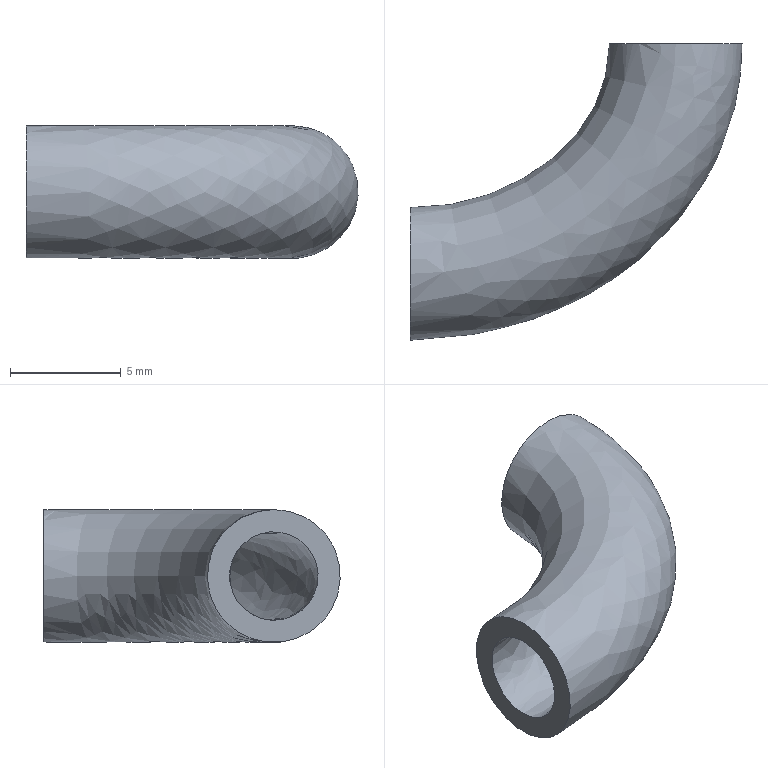Part | NX | features solid 2 | 1 solid | 4 faces | box 15.025 x 13.395 x 6 mm | volume 276.383 mm3 | plane 2 | spline 2